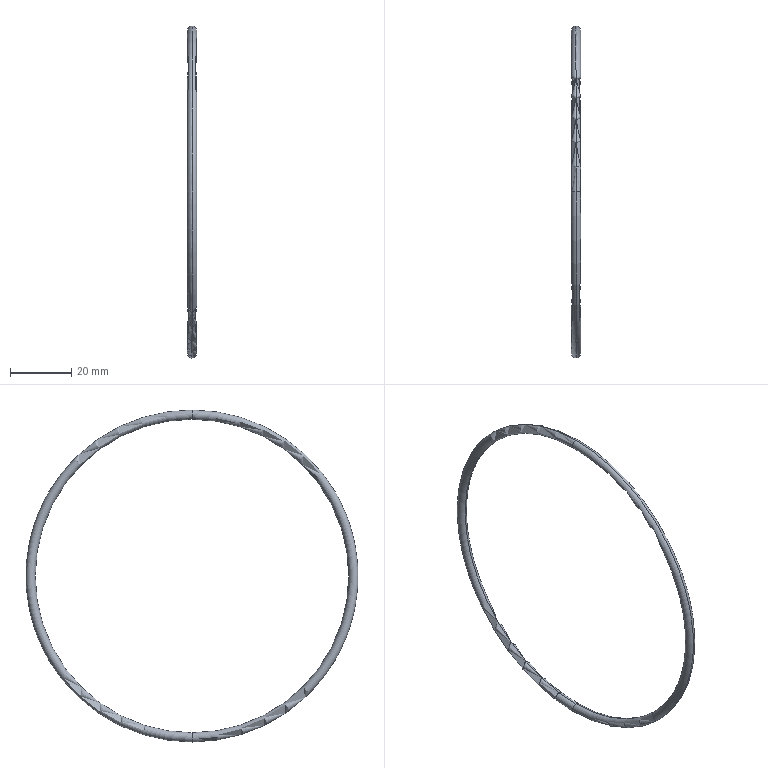Part | SolidWorks | features BaseBody 1 | 1 solid | 4 faces | box 3 x 108 x 108 mm | volume 2332 mm3 | torus 4
STEP:
#1=CARTESIAN_POINT('',(-8.,0.,-54.));
#2=VERTEX_POINT('',#1);
#3=CARTESIAN_POINT('',(-8.,0.,-51.));
#4=VERTEX_POINT('',#3);
#5=CARTESIAN_POINT('',(-8.,0.,-52.5));
#6=DIRECTION('',(0.,-1.,0.));
#7=DIRECTION('',(1.,0.,0.));
#8=AXIS2_PLACEMENT_3D('',#5,#6,#7);
#9=CIRCLE('',#8,1.5);
#10=EDGE_CURVE('',#2,#4,#9,.T.);
#11=ORIENTED_EDGE('',*,*,#10,.F.);
#12=CARTESIAN_POINT('',(-8.,0.,54.));
#13=VERTEX_POINT('',#12);
#14=CARTESIAN_POINT('',(-8.,0.,0.));
#15=DIRECTION('',(1.,0.,0.));
#16=DIRECTION('',(0.,1.,0.));
#17=AXIS2_PLACEMENT_3D('',#14,#15,#16);
#18=CIRCLE('',#17,54.);
#19=EDGE_CURVE('',#2,#13,#18,.T.);
#20=ORIENTED_EDGE('',*,*,#19,.T.);
#21=CARTESIAN_POINT('',(-8.,0.,51.));
#22=VERTEX_POINT('',#21);
#23=CARTESIAN_POINT('',(-8.,0.,52.5));
#24=DIRECTION('',(0.,1.,0.));
#25=DIRECTION('',(-1.,0.,0.));
#26=AXIS2_PLACEMENT_3D('',#23,#24,#25);
#27=CIRCLE('',#26,1.5);
#28=EDGE_CURVE('',#13,#22,#27,.T.);
#29=ORIENTED_EDGE('',*,*,#28,.T.);
#30=CARTESIAN_POINT('',(-8.,0.,0.));
#31=DIRECTION('',(1.,0.,0.));
#32=DIRECTION('',(0.,1.,0.));
#33=AXIS2_PLACEMENT_3D('',#30,#31,#32);
#34=CIRCLE('',#33,51.);
#35=EDGE_CURVE('',#4,#22,#34,.T.);
#36=ORIENTED_EDGE('',*,*,#35,.F.);
#37=EDGE_LOOP('',(#11,#20,#29,#36));
#38=FACE_OUTER_BOUND('',#37,.T.);
#39=CARTESIAN_POINT('',(-8.,0.,0.));
#40=DIRECTION('',(1.,0.,0.));
#41=DIRECTION('',(0.,0.,1.));
#42=AXIS2_PLACEMENT_3D('',#39,#40,#41);
#43=TOROIDAL_SURFACE('',#42,52.5,1.5);
#44=ADVANCED_FACE('',(#38),#43,.T.);
#45=ORIENTED_EDGE('',*,*,#28,.F.);
#46=CARTESIAN_POINT('',(-8.,0.,0.));
#47=DIRECTION('',(1.,0.,0.));
#48=DIRECTION('',(0.,1.,0.));
#49=AXIS2_PLACEMENT_3D('',#46,#47,#48);
#50=CIRCLE('',#49,54.);
#51=EDGE_CURVE('',#13,#2,#50,.T.);
#52=ORIENTED_EDGE('',*,*,#51,.T.);
#53=ORIENTED_EDGE('',*,*,#10,.T.);
#54=CARTESIAN_POINT('',(-8.,0.,0.));
#55=DIRECTION('',(1.,0.,0.));
#56=DIRECTION('',(0.,1.,0.));
#57=AXIS2_PLACEMENT_3D('',#54,#55,#56);
#58=CIRCLE('',#57,51.);
#59=EDGE_CURVE('',#22,#4,#58,.T.);
#60=ORIENTED_EDGE('',*,*,#59,.F.);
#61=EDGE_LOOP('',(#45,#52,#53,#60));
#62=FACE_OUTER_BOUND('',#61,.T.);
#63=CARTESIAN_POINT('',(-8.,0.,0.));
#64=DIRECTION('',(1.,0.,0.));
#65=DIRECTION('',(0.,0.,1.));
#66=AXIS2_PLACEMENT_3D('',#63,#64,#65);
#67=TOROIDAL_SURFACE('',#66,52.5,1.5);
#68=ADVANCED_FACE('',(#62),#67,.T.);
#69=ORIENTED_EDGE('',*,*,#51,.F.);
#70=CARTESIAN_POINT('',(-8.,0.,52.5));
#71=DIRECTION('',(0.,1.,0.));
#72=DIRECTION('',(-1.,0.,0.));
#73=AXIS2_PLACEMENT_3D('',#70,#71,#72);
#74=CIRCLE('',#73,1.5);
#75=EDGE_CURVE('',#22,#13,#74,.T.);
#76=ORIENTED_EDGE('',*,*,#75,.F.);
#77=ORIENTED_EDGE('',*,*,#59,.T.);
#78=CARTESIAN_POINT('',(-8.,0.,-52.5));
#79=DIRECTION('',(0.,-1.,0.));
#80=DIRECTION('',(1.,0.,0.));
#81=AXIS2_PLACEMENT_3D('',#78,#79,#80);
#82=CIRCLE('',#81,1.5);
#83=EDGE_CURVE('',#4,#2,#82,.T.);
#84=ORIENTED_EDGE('',*,*,#83,.T.);
#85=EDGE_LOOP('',(#69,#76,#77,#84));
#86=FACE_OUTER_BOUND('',#85,.T.);
#87=CARTESIAN_POINT('',(-8.,0.,0.));
#88=DIRECTION('',(1.,0.,0.));
#89=DIRECTION('',(0.,0.,1.));
#90=AXIS2_PLACEMENT_3D('',#87,#88,#89);
#91=TOROIDAL_SURFACE('',#90,52.5,1.5);
#92=ADVANCED_FACE('',(#86),#91,.T.);
#93=ORIENTED_EDGE('',*,*,#19,.F.);
#94=ORIENTED_EDGE('',*,*,#83,.F.);
#95=ORIENTED_EDGE('',*,*,#35,.T.);
#96=ORIENTED_EDGE('',*,*,#75,.T.);
#97=EDGE_LOOP('',(#93,#94,#95,#96));
#98=FACE_OUTER_BOUND('',#97,.T.);
#99=CARTESIAN_POINT('',(-8.,0.,0.));
#100=DIRECTION('',(1.,0.,0.));
#101=DIRECTION('',(0.,0.,1.));
#102=AXIS2_PLACEMENT_3D('',#99,#100,#101);
#103=TOROIDAL_SURFACE('',#102,52.5,1.5);
#104=ADVANCED_FACE('',(#98),#103,.T.);
#105=CLOSED_SHELL('',(#44,#68,#92,#104));
#106=MANIFOLD_SOLID_BREP('',#105);
#107=CARTESIAN_POINT('',(0.,0.,0.));
#108=DIRECTION('',(0.,0.,1.));
#109=DIRECTION('',(1.,0.,0.));
#110=AXIS2_PLACEMENT_3D('',#107,#108,#109);
#111=(LENGTH_UNIT()NAMED_UNIT(*)SI_UNIT(.MILLI.,.METRE.));
#112=UNCERTAINTY_MEASURE_WITH_UNIT(LENGTH_MEASURE(0.00001),#111,'','');
#113=(NAMED_UNIT(*)PLANE_ANGLE_UNIT()SI_UNIT($,.RADIAN.));
#114=(NAMED_UNIT(*)SI_UNIT($,.STERADIAN.)SOLID_ANGLE_UNIT());
#115=(GEOMETRIC_REPRESENTATION_CONTEXT(3)GLOBAL_UNCERTAINTY_ASSIGNED_CONTEXT((#112))GLOBAL_UNIT_ASSIGNED_CONTEXT((#111,#113,#114))REPRESENTATION_CONTEXT('',''));
#116=ADVANCED_BREP_SHAPE_REPRESENTATION('',(#106,#110),#115);